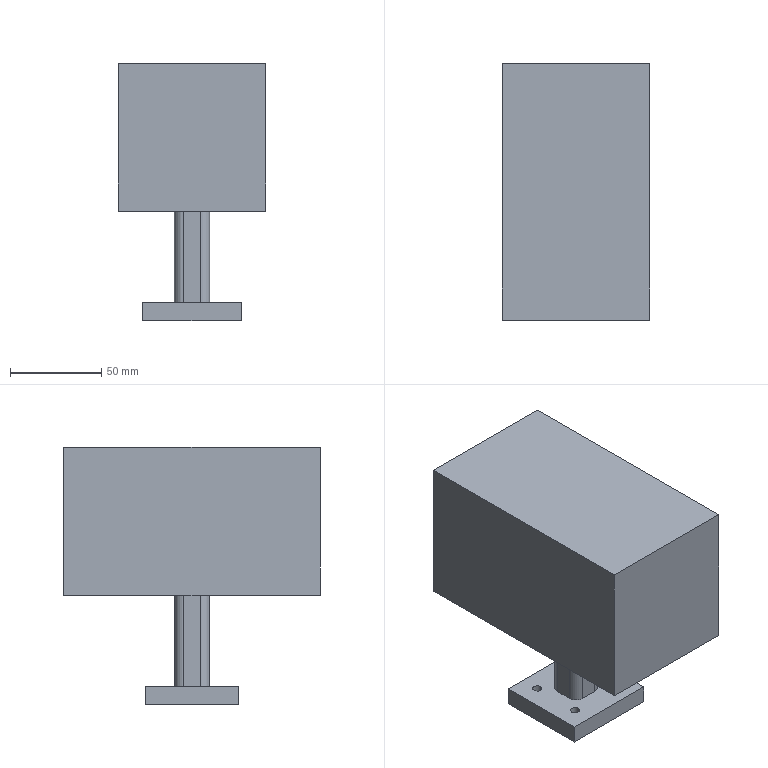Part | SolidWorks | features SplitBody 1 | 1 solid | 55 faces | box 80.791 x 140.331 x 141 mm | volume 119949 mm3 | plane 31 | cylinder 24 | commonest cylinder face diameters 5 x8 9 x8 6 x4 10 x4